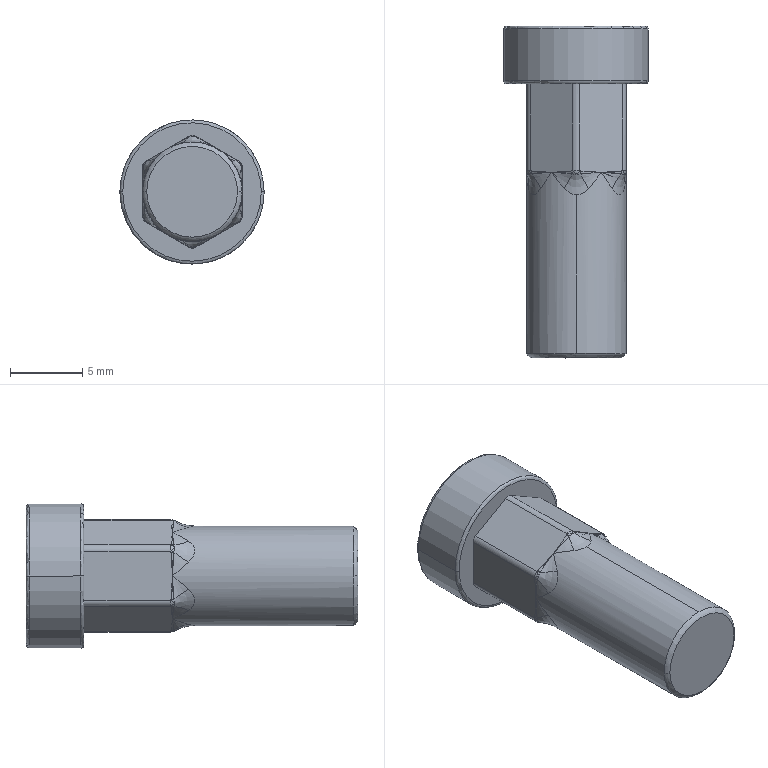Part | NX | features BREP 1 | 1 solid | 130 faces | box 10.002 x 23.005 x 10.001 mm | volume 588.706 mm3 | spline 76 | plane 24 | cylinder 16 | torus 6 | sphere 6 | cone 2 | commonest cylinder face diameters 1 x7 5 x3 6.1 x2 6.9 x2 10 x2